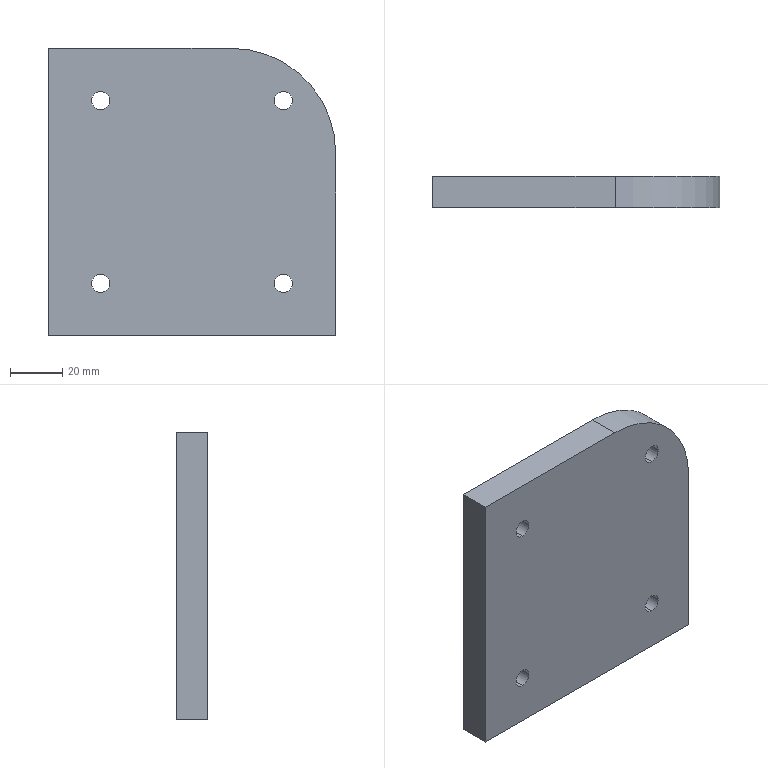Part | 1 solid | 15 faces | box 110 x 12 x 110 mm | volume 139232 mm3 | cylinder 9 | plane 6 | commonest cylinder face diameters 7 x8 80 x1
STEP:
#1=CARTESIAN_POINT('',(328.,-10.,546.5));
#2=VERTEX_POINT('',#1);
#3=CARTESIAN_POINT('',(328.,-10.,553.5));
#4=VERTEX_POINT('',#3);
#5=CARTESIAN_POINT('',(328.,-10.,550.));
#6=DIRECTION('',(0.,1.,0.));
#7=DIRECTION('',(0.,0.,1.));
#8=AXIS2_PLACEMENT_3D('',#5,#6,#7);
#9=CIRCLE('',#8,3.5);
#10=EDGE_CURVE('',#2,#4,#9,.T.);
#11=ORIENTED_EDGE('',*,*,#10,.F.);
#12=CARTESIAN_POINT('',(328.,2.,546.5));
#13=VERTEX_POINT('',#12);
#14=CARTESIAN_POINT('',(328.,-10.,546.5));
#15=DIRECTION('',(0.,1.,0.));
#16=VECTOR('',#15,1000.);
#17=LINE('',#14,#16);
#18=EDGE_CURVE('',#2,#13,#17,.T.);
#19=ORIENTED_EDGE('',*,*,#18,.T.);
#20=CARTESIAN_POINT('',(328.,2.,553.5));
#21=VERTEX_POINT('',#20);
#22=CARTESIAN_POINT('',(328.,2.,550.));
#23=DIRECTION('',(0.,-1.,0.));
#24=DIRECTION('',(0.,0.,1.));
#25=AXIS2_PLACEMENT_3D('',#22,#23,#24);
#26=CIRCLE('',#25,3.5);
#27=EDGE_CURVE('',#21,#13,#26,.T.);
#28=ORIENTED_EDGE('',*,*,#27,.F.);
#29=CARTESIAN_POINT('',(328.,-10.,553.5));
#30=DIRECTION('',(0.,1.,0.));
#31=VECTOR('',#30,1000.);
#32=LINE('',#29,#31);
#33=EDGE_CURVE('',#4,#21,#32,.T.);
#34=ORIENTED_EDGE('',*,*,#33,.F.);
#35=EDGE_LOOP('',(#11,#19,#28,#34));
#36=FACE_OUTER_BOUND('',#35,.T.);
#37=CARTESIAN_POINT('',(328.,-10.,550.));
#38=DIRECTION('',(0.,1.,0.));
#39=DIRECTION('',(0.,0.,1.));
#40=AXIS2_PLACEMENT_3D('',#37,#38,#39);
#41=CYLINDRICAL_SURFACE('',#40,3.5);
#42=ADVANCED_FACE('',(#36),#41,.F.);
#43=CARTESIAN_POINT('',(398.,-10.,546.5));
#44=VERTEX_POINT('',#43);
#45=CARTESIAN_POINT('',(398.,-10.,553.5));
#46=VERTEX_POINT('',#45);
#47=CARTESIAN_POINT('',(398.,-10.,550.));
#48=DIRECTION('',(0.,1.,0.));
#49=DIRECTION('',(0.,0.,1.));
#50=AXIS2_PLACEMENT_3D('',#47,#48,#49);
#51=CIRCLE('',#50,3.5);
#52=EDGE_CURVE('',#44,#46,#51,.T.);
#53=ORIENTED_EDGE('',*,*,#52,.F.);
#54=CARTESIAN_POINT('',(398.,2.,546.5));
#55=VERTEX_POINT('',#54);
#56=CARTESIAN_POINT('',(398.,-10.,546.5));
#57=DIRECTION('',(0.,1.,0.));
#58=VECTOR('',#57,1000.);
#59=LINE('',#56,#58);
#60=EDGE_CURVE('',#44,#55,#59,.T.);
#61=ORIENTED_EDGE('',*,*,#60,.T.);
#62=CARTESIAN_POINT('',(398.,2.,553.5));
#63=VERTEX_POINT('',#62);
#64=CARTESIAN_POINT('',(398.,2.,550.));
#65=DIRECTION('',(0.,-1.,0.));
#66=DIRECTION('',(0.,0.,1.));
#67=AXIS2_PLACEMENT_3D('',#64,#65,#66);
#68=CIRCLE('',#67,3.5);
#69=EDGE_CURVE('',#63,#55,#68,.T.);
#70=ORIENTED_EDGE('',*,*,#69,.F.);
#71=CARTESIAN_POINT('',(398.,-10.,553.5));
#72=DIRECTION('',(0.,1.,0.));
#73=VECTOR('',#72,1000.);
#74=LINE('',#71,#73);
#75=EDGE_CURVE('',#46,#63,#74,.T.);
#76=ORIENTED_EDGE('',*,*,#75,.F.);
#77=EDGE_LOOP('',(#53,#61,#70,#76));
#78=FACE_OUTER_BOUND('',#77,.T.);
#79=CARTESIAN_POINT('',(398.,-10.,550.));
#80=DIRECTION('',(0.,1.,0.));
#81=DIRECTION('',(0.,0.,1.));
#82=AXIS2_PLACEMENT_3D('',#79,#80,#81);
#83=CYLINDRICAL_SURFACE('',#82,3.5);
#84=ADVANCED_FACE('',(#78),#83,.F.);
#85=CARTESIAN_POINT('',(398.,-10.,616.5));
#86=VERTEX_POINT('',#85);
#87=CARTESIAN_POINT('',(398.,-10.,623.5));
#88=VERTEX_POINT('',#87);
#89=CARTESIAN_POINT('',(398.,-10.,620.));
#90=DIRECTION('',(0.,1.,0.));
#91=DIRECTION('',(0.,0.,1.));
#92=AXIS2_PLACEMENT_3D('',#89,#90,#91);
#93=CIRCLE('',#92,3.5);
#94=EDGE_CURVE('',#86,#88,#93,.T.);
#95=ORIENTED_EDGE('',*,*,#94,.F.);
#96=CARTESIAN_POINT('',(398.,2.,616.5));
#97=VERTEX_POINT('',#96);
#98=CARTESIAN_POINT('',(398.,-10.,616.5));
#99=DIRECTION('',(0.,1.,0.));
#100=VECTOR('',#99,1000.);
#101=LINE('',#98,#100);
#102=EDGE_CURVE('',#86,#97,#101,.T.);
#103=ORIENTED_EDGE('',*,*,#102,.T.);
#104=CARTESIAN_POINT('',(398.,2.,623.5));
#105=VERTEX_POINT('',#104);
#106=CARTESIAN_POINT('',(398.,2.,620.));
#107=DIRECTION('',(0.,-1.,0.));
#108=DIRECTION('',(0.,0.,1.));
#109=AXIS2_PLACEMENT_3D('',#106,#107,#108);
#110=CIRCLE('',#109,3.5);
#111=EDGE_CURVE('',#105,#97,#110,.T.);
#112=ORIENTED_EDGE('',*,*,#111,.F.);
#113=CARTESIAN_POINT('',(398.,-10.,623.5));
#114=DIRECTION('',(0.,1.,0.));
#115=VECTOR('',#114,1000.);
#116=LINE('',#113,#115);
#117=EDGE_CURVE('',#88,#105,#116,.T.);
#118=ORIENTED_EDGE('',*,*,#117,.F.);
#119=EDGE_LOOP('',(#95,#103,#112,#118));
#120=FACE_OUTER_BOUND('',#119,.T.);
#121=CARTESIAN_POINT('',(398.,-10.,620.));
#122=DIRECTION('',(0.,1.,0.));
#123=DIRECTION('',(0.,0.,1.));
#124=AXIS2_PLACEMENT_3D('',#121,#122,#123);
#125=CYLINDRICAL_SURFACE('',#124,3.5);
#126=ADVANCED_FACE('',(#120),#125,.F.);
#127=CARTESIAN_POINT('',(328.,-10.,616.5));
#128=VERTEX_POINT('',#127);
#129=CARTESIAN_POINT('',(328.,-10.,623.5));
#130=VERTEX_POINT('',#129);
#131=CARTESIAN_POINT('',(328.,-10.,620.));
#132=DIRECTION('',(0.,1.,0.));
#133=DIRECTION('',(0.,0.,1.));
#134=AXIS2_PLACEMENT_3D('',#131,#132,#133);
#135=CIRCLE('',#134,3.5);
#136=EDGE_CURVE('',#128,#130,#135,.T.);
#137=ORIENTED_EDGE('',*,*,#136,.F.);
#138=CARTESIAN_POINT('',(328.,2.,616.5));
#139=VERTEX_POINT('',#138);
#140=CARTESIAN_POINT('',(328.,-10.,616.5));
#141=DIRECTION('',(0.,1.,0.));
#142=VECTOR('',#141,1000.);
#143=LINE('',#140,#142);
#144=EDGE_CURVE('',#128,#139,#143,.T.);
#145=ORIENTED_EDGE('',*,*,#144,.T.);
#146=CARTESIAN_POINT('',(328.,2.,623.5));
#147=VERTEX_POINT('',#146);
#148=CARTESIAN_POINT('',(328.,2.,620.));
#149=DIRECTION('',(0.,-1.,0.));
#150=DIRECTION('',(0.,0.,1.));
#151=AXIS2_PLACEMENT_3D('',#148,#149,#150);
#152=CIRCLE('',#151,3.5);
#153=EDGE_CURVE('',#147,#139,#152,.T.);
#154=ORIENTED_EDGE('',*,*,#153,.F.);
#155=CARTESIAN_POINT('',(328.,-10.,623.5));
#156=DIRECTION('',(0.,1.,0.));
#157=VECTOR('',#156,1000.);
#158=LINE('',#155,#157);
#159=EDGE_CURVE('',#130,#147,#158,.T.);
#160=ORIENTED_EDGE('',*,*,#159,.F.);
#161=EDGE_LOOP('',(#137,#145,#154,#160));
#162=FACE_OUTER_BOUND('',#161,.T.);
#163=CARTESIAN_POINT('',(328.,-10.,620.));
#164=DIRECTION('',(0.,1.,0.));
#165=DIRECTION('',(0.,0.,1.));
#166=AXIS2_PLACEMENT_3D('',#163,#164,#165);
#167=CYLINDRICAL_SURFACE('',#166,3.5);
#168=ADVANCED_FACE('',(#162),#167,.F.);
#169=CARTESIAN_POINT('',(328.,-10.,550.));
#170=DIRECTION('',(0.,1.,0.));
#171=DIRECTION('',(0.,0.,1.));
#172=AXIS2_PLACEMENT_3D('',#169,#170,#171);
#173=CIRCLE('',#172,3.5);
#174=EDGE_CURVE('',#4,#2,#173,.T.);
#175=ORIENTED_EDGE('',*,*,#174,.T.);
#176=ORIENTED_EDGE('',*,*,#10,.T.);
#177=EDGE_LOOP('',(#175,#176));
#178=FACE_BOUND('',#177,.T.);
#179=CARTESIAN_POINT('',(398.,-10.,550.));
#180=DIRECTION('',(0.,1.,0.));
#181=DIRECTION('',(0.,0.,1.));
#182=AXIS2_PLACEMENT_3D('',#179,#180,#181);
#183=CIRCLE('',#182,3.5);
#184=EDGE_CURVE('',#46,#44,#183,.T.);
#185=ORIENTED_EDGE('',*,*,#184,.T.);
#186=ORIENTED_EDGE('',*,*,#52,.T.);
#187=EDGE_LOOP('',(#185,#186));
#188=FACE_BOUND('',#187,.T.);
#189=CARTESIAN_POINT('',(398.,-10.,620.));
#190=DIRECTION('',(0.,1.,0.));
#191=DIRECTION('',(0.,0.,1.));
#192=AXIS2_PLACEMENT_3D('',#189,#190,#191);
#193=CIRCLE('',#192,3.5);
#194=EDGE_CURVE('',#88,#86,#193,.T.);
#195=ORIENTED_EDGE('',*,*,#194,.T.);
#196=ORIENTED_EDGE('',*,*,#94,.T.);
#197=EDGE_LOOP('',(#195,#196));
#198=FACE_BOUND('',#197,.T.);
#199=CARTESIAN_POINT('',(328.,-10.,620.));
#200=DIRECTION('',(0.,1.,0.));
#201=DIRECTION('',(0.,0.,1.));
#202=AXIS2_PLACEMENT_3D('',#199,#200,#201);
#203=CIRCLE('',#202,3.5);
#204=EDGE_CURVE('',#130,#128,#203,.T.);
#205=ORIENTED_EDGE('',*,*,#204,.T.);
#206=ORIENTED_EDGE('',*,*,#136,.T.);
#207=EDGE_LOOP('',(#205,#206));
#208=FACE_BOUND('',#207,.T.);
#209=CARTESIAN_POINT('',(308.,-10.,640.));
#210=VERTEX_POINT('',#209);
#211=CARTESIAN_POINT('',(308.,-10.,530.));
#212=VERTEX_POINT('',#211);
#213=CARTESIAN_POINT('',(308.,-10.,80.));
#214=DIRECTION('',(0.,0.,-1.));
#215=VECTOR('',#214,1000.);
#216=LINE('',#213,#215);
#217=EDGE_CURVE('',#210,#212,#216,.T.);
#218=ORIENTED_EDGE('',*,*,#217,.T.);
#219=CARTESIAN_POINT('',(418.,-10.,530.));
#220=VERTEX_POINT('',#219);
#221=CARTESIAN_POINT('',(18.,-10.,530.));
#222=DIRECTION('',(1.,0.,0.));
#223=VECTOR('',#222,1000.);
#224=LINE('',#221,#223);
#225=EDGE_CURVE('',#212,#220,#224,.T.);
#226=ORIENTED_EDGE('',*,*,#225,.T.);
#227=CARTESIAN_POINT('',(418.,-10.,600.));
#228=VERTEX_POINT('',#227);
#229=CARTESIAN_POINT('',(418.,-10.,80.));
#230=DIRECTION('',(0.,0.,1.));
#231=VECTOR('',#230,1000.);
#232=LINE('',#229,#231);
#233=EDGE_CURVE('',#220,#228,#232,.T.);
#234=ORIENTED_EDGE('',*,*,#233,.T.);
#235=CARTESIAN_POINT('',(378.,-10.,640.));
#236=VERTEX_POINT('',#235);
#237=CARTESIAN_POINT('',(378.,-10.,600.));
#238=DIRECTION('',(0.,-1.,0.));
#239=DIRECTION('',(0.,0.,1.));
#240=AXIS2_PLACEMENT_3D('',#237,#238,#239);
#241=CIRCLE('',#240,40.);
#242=EDGE_CURVE('',#228,#236,#241,.T.);
#243=ORIENTED_EDGE('',*,*,#242,.T.);
#244=CARTESIAN_POINT('',(18.,-10.,640.));
#245=DIRECTION('',(-1.,0.,0.));
#246=VECTOR('',#245,1000.);
#247=LINE('',#244,#246);
#248=EDGE_CURVE('',#236,#210,#247,.T.);
#249=ORIENTED_EDGE('',*,*,#248,.T.);
#250=EDGE_LOOP('',(#218,#226,#234,#243,#249));
#251=FACE_OUTER_BOUND('',#250,.T.);
#252=CARTESIAN_POINT('',(18.,-10.,80.));
#253=DIRECTION('',(0.,-1.,0.));
#254=DIRECTION('',(0.,0.,-1.));
#255=AXIS2_PLACEMENT_3D('',#252,#253,#254);
#256=PLANE('',#255);
#257=ADVANCED_FACE('',(#178,#188,#198,#208,#251),#256,.T.);
#258=ORIENTED_EDGE('',*,*,#18,.F.);
#259=ORIENTED_EDGE('',*,*,#174,.F.);
#260=ORIENTED_EDGE('',*,*,#33,.T.);
#261=CARTESIAN_POINT('',(328.,2.,550.));
#262=DIRECTION('',(0.,-1.,0.));
#263=DIRECTION('',(0.,0.,1.));
#264=AXIS2_PLACEMENT_3D('',#261,#262,#263);
#265=CIRCLE('',#264,3.5);
#266=EDGE_CURVE('',#13,#21,#265,.T.);
#267=ORIENTED_EDGE('',*,*,#266,.F.);
#268=EDGE_LOOP('',(#258,#259,#260,#267));
#269=FACE_OUTER_BOUND('',#268,.T.);
#270=CARTESIAN_POINT('',(328.,-10.,550.));
#271=DIRECTION('',(0.,1.,0.));
#272=DIRECTION('',(0.,0.,1.));
#273=AXIS2_PLACEMENT_3D('',#270,#271,#272);
#274=CYLINDRICAL_SURFACE('',#273,3.5);
#275=ADVANCED_FACE('',(#269),#274,.F.);
#276=ORIENTED_EDGE('',*,*,#60,.F.);
#277=ORIENTED_EDGE('',*,*,#184,.F.);
#278=ORIENTED_EDGE('',*,*,#75,.T.);
#279=CARTESIAN_POINT('',(398.,2.,550.));
#280=DIRECTION('',(0.,-1.,0.));
#281=DIRECTION('',(0.,0.,1.));
#282=AXIS2_PLACEMENT_3D('',#279,#280,#281);
#283=CIRCLE('',#282,3.5);
#284=EDGE_CURVE('',#55,#63,#283,.T.);
#285=ORIENTED_EDGE('',*,*,#284,.F.);
#286=EDGE_LOOP('',(#276,#277,#278,#285));
#287=FACE_OUTER_BOUND('',#286,.T.);
#288=CARTESIAN_POINT('',(398.,-10.,550.));
#289=DIRECTION('',(0.,1.,0.));
#290=DIRECTION('',(0.,0.,1.));
#291=AXIS2_PLACEMENT_3D('',#288,#289,#290);
#292=CYLINDRICAL_SURFACE('',#291,3.5);
#293=ADVANCED_FACE('',(#287),#292,.F.);
#294=ORIENTED_EDGE('',*,*,#102,.F.);
#295=ORIENTED_EDGE('',*,*,#194,.F.);
#296=ORIENTED_EDGE('',*,*,#117,.T.);
#297=CARTESIAN_POINT('',(398.,2.,620.));
#298=DIRECTION('',(0.,-1.,0.));
#299=DIRECTION('',(0.,0.,1.));
#300=AXIS2_PLACEMENT_3D('',#297,#298,#299);
#301=CIRCLE('',#300,3.5);
#302=EDGE_CURVE('',#97,#105,#301,.T.);
#303=ORIENTED_EDGE('',*,*,#302,.F.);
#304=EDGE_LOOP('',(#294,#295,#296,#303));
#305=FACE_OUTER_BOUND('',#304,.T.);
#306=CARTESIAN_POINT('',(398.,-10.,620.));
#307=DIRECTION('',(0.,1.,0.));
#308=DIRECTION('',(0.,0.,1.));
#309=AXIS2_PLACEMENT_3D('',#306,#307,#308);
#310=CYLINDRICAL_SURFACE('',#309,3.5);
#311=ADVANCED_FACE('',(#305),#310,.F.);
#312=ORIENTED_EDGE('',*,*,#144,.F.);
#313=ORIENTED_EDGE('',*,*,#204,.F.);
#314=ORIENTED_EDGE('',*,*,#159,.T.);
#315=CARTESIAN_POINT('',(328.,2.,620.));
#316=DIRECTION('',(0.,-1.,0.));
#317=DIRECTION('',(0.,0.,1.));
#318=AXIS2_PLACEMENT_3D('',#315,#316,#317);
#319=CIRCLE('',#318,3.5);
#320=EDGE_CURVE('',#139,#147,#319,.T.);
#321=ORIENTED_EDGE('',*,*,#320,.F.);
#322=EDGE_LOOP('',(#312,#313,#314,#321));
#323=FACE_OUTER_BOUND('',#322,.T.);
#324=CARTESIAN_POINT('',(328.,-10.,620.));
#325=DIRECTION('',(0.,1.,0.));
#326=DIRECTION('',(0.,0.,1.));
#327=AXIS2_PLACEMENT_3D('',#324,#325,#326);
#328=CYLINDRICAL_SURFACE('',#327,3.5);
#329=ADVANCED_FACE('',(#323),#328,.F.);
#330=ORIENTED_EDGE('',*,*,#225,.F.);
#331=CARTESIAN_POINT('',(308.,2.,530.));
#332=VERTEX_POINT('',#331);
#333=CARTESIAN_POINT('',(308.,0.,530.));
#334=DIRECTION('',(0.,1.,0.));
#335=VECTOR('',#334,1000.);
#336=LINE('',#333,#335);
#337=EDGE_CURVE('',#212,#332,#336,.T.);
#338=ORIENTED_EDGE('',*,*,#337,.T.);
#339=CARTESIAN_POINT('',(418.,2.,530.));
#340=VERTEX_POINT('',#339);
#341=CARTESIAN_POINT('',(308.,2.,530.));
#342=DIRECTION('',(1.,0.,0.));
#343=VECTOR('',#342,1000.);
#344=LINE('',#341,#343);
#345=EDGE_CURVE('',#332,#340,#344,.T.);
#346=ORIENTED_EDGE('',*,*,#345,.T.);
#347=CARTESIAN_POINT('',(418.,0.,530.));
#348=DIRECTION('',(0.,-1.,0.));
#349=VECTOR('',#348,1000.);
#350=LINE('',#347,#349);
#351=EDGE_CURVE('',#340,#220,#350,.T.);
#352=ORIENTED_EDGE('',*,*,#351,.T.);
#353=EDGE_LOOP('',(#330,#338,#346,#352));
#354=FACE_OUTER_BOUND('',#353,.T.);
#355=CARTESIAN_POINT('',(308.,0.,530.));
#356=DIRECTION('',(0.,0.,-1.));
#357=DIRECTION('',(-1.,0.,0.));
#358=AXIS2_PLACEMENT_3D('',#355,#356,#357);
#359=PLANE('',#358);
#360=ADVANCED_FACE('',(#354),#359,.T.);
#361=ORIENTED_EDGE('',*,*,#217,.F.);
#362=CARTESIAN_POINT('',(308.,2.,640.));
#363=VERTEX_POINT('',#362);
#364=CARTESIAN_POINT('',(308.,0.,640.));
#365=DIRECTION('',(0.,1.,0.));
#366=VECTOR('',#365,1000.);
#367=LINE('',#364,#366);
#368=EDGE_CURVE('',#210,#363,#367,.T.);
#369=ORIENTED_EDGE('',*,*,#368,.T.);
#370=CARTESIAN_POINT('',(308.,2.,-150.));
#371=DIRECTION('',(0.,0.,-1.));
#372=VECTOR('',#371,1000.);
#373=LINE('',#370,#372);
#374=EDGE_CURVE('',#363,#332,#373,.T.);
#375=ORIENTED_EDGE('',*,*,#374,.T.);
#376=ORIENTED_EDGE('',*,*,#337,.F.);
#377=EDGE_LOOP('',(#361,#369,#375,#376));
#378=FACE_OUTER_BOUND('',#377,.T.);
#379=CARTESIAN_POINT('',(308.,0.,-150.));
#380=DIRECTION('',(-1.,0.,0.));
#381=DIRECTION('',(0.,0.,1.));
#382=AXIS2_PLACEMENT_3D('',#379,#380,#381);
#383=PLANE('',#382);
#384=ADVANCED_FACE('',(#378),#383,.T.);
#385=CARTESIAN_POINT('',(378.,2.,640.));
#386=VERTEX_POINT('',#385);
#387=CARTESIAN_POINT('',(378.,-10.,640.));
#388=DIRECTION('',(0.,-1.,0.));
#389=VECTOR('',#388,1000.);
#390=LINE('',#387,#389);
#391=EDGE_CURVE('',#386,#236,#390,.T.);
#392=ORIENTED_EDGE('',*,*,#391,.F.);
#393=CARTESIAN_POINT('',(418.,2.,640.));
#394=DIRECTION('',(1.,0.,0.));
#395=VECTOR('',#394,1000.);
#396=LINE('',#393,#395);
#397=EDGE_CURVE('',#363,#386,#396,.T.);
#398=ORIENTED_EDGE('',*,*,#397,.F.);
#399=ORIENTED_EDGE('',*,*,#368,.F.);
#400=ORIENTED_EDGE('',*,*,#248,.F.);
#401=EDGE_LOOP('',(#392,#398,#399,#400));
#402=FACE_OUTER_BOUND('',#401,.T.);
#403=CARTESIAN_POINT('',(418.,-10.,640.));
#404=DIRECTION('',(0.,0.,-1.));
#405=DIRECTION('',(-1.,0.,0.));
#406=AXIS2_PLACEMENT_3D('',#403,#404,#405);
#407=PLANE('',#406);
#408=ADVANCED_FACE('',(#402),#407,.F.);
#409=ORIENTED_EDGE('',*,*,#242,.F.);
#410=CARTESIAN_POINT('',(418.,2.,600.));
#411=VERTEX_POINT('',#410);
#412=CARTESIAN_POINT('',(418.,-10.,600.));
#413=DIRECTION('',(0.,1.,0.));
#414=VECTOR('',#413,1000.);
#415=LINE('',#412,#414);
#416=EDGE_CURVE('',#228,#411,#415,.T.);
#417=ORIENTED_EDGE('',*,*,#416,.T.);
#418=CARTESIAN_POINT('',(378.,2.,600.));
#419=DIRECTION('',(0.,-1.,0.));
#420=DIRECTION('',(0.,0.,1.));
#421=AXIS2_PLACEMENT_3D('',#418,#419,#420);
#422=CIRCLE('',#421,40.);
#423=EDGE_CURVE('',#411,#386,#422,.T.);
#424=ORIENTED_EDGE('',*,*,#423,.T.);
#425=ORIENTED_EDGE('',*,*,#391,.T.);
#426=EDGE_LOOP('',(#409,#417,#424,#425));
#427=FACE_OUTER_BOUND('',#426,.T.);
#428=CARTESIAN_POINT('',(378.,-10.,600.));
#429=DIRECTION('',(0.,1.,0.));
#430=DIRECTION('',(0.,0.,1.));
#431=AXIS2_PLACEMENT_3D('',#428,#429,#430);
#432=CYLINDRICAL_SURFACE('',#431,40.);
#433=ADVANCED_FACE('',(#427),#432,.T.);
#434=CARTESIAN_POINT('',(418.,2.,640.));
#435=DIRECTION('',(0.,0.,-1.));
#436=VECTOR('',#435,1000.);
#437=LINE('',#434,#436);
#438=EDGE_CURVE('',#411,#340,#437,.T.);
#439=ORIENTED_EDGE('',*,*,#438,.F.);
#440=ORIENTED_EDGE('',*,*,#416,.F.);
#441=ORIENTED_EDGE('',*,*,#233,.F.);
#442=ORIENTED_EDGE('',*,*,#351,.F.);
#443=EDGE_LOOP('',(#439,#440,#441,#442));
#444=FACE_OUTER_BOUND('',#443,.T.);
#445=CARTESIAN_POINT('',(418.,-10.,640.));
#446=DIRECTION('',(-1.,0.,0.));
#447=DIRECTION('',(0.,0.,1.));
#448=AXIS2_PLACEMENT_3D('',#445,#446,#447);
#449=PLANE('',#448);
#450=ADVANCED_FACE('',(#444),#449,.F.);
#451=ORIENTED_EDGE('',*,*,#27,.T.);
#452=ORIENTED_EDGE('',*,*,#266,.T.);
#453=EDGE_LOOP('',(#451,#452));
#454=FACE_BOUND('',#453,.T.);
#455=ORIENTED_EDGE('',*,*,#69,.T.);
#456=ORIENTED_EDGE('',*,*,#284,.T.);
#457=EDGE_LOOP('',(#455,#456));
#458=FACE_BOUND('',#457,.T.);
#459=ORIENTED_EDGE('',*,*,#111,.T.);
#460=ORIENTED_EDGE('',*,*,#302,.T.);
#461=EDGE_LOOP('',(#459,#460));
#462=FACE_BOUND('',#461,.T.);
#463=ORIENTED_EDGE('',*,*,#153,.T.);
#464=ORIENTED_EDGE('',*,*,#320,.T.);
#465=EDGE_LOOP('',(#463,#464));
#466=FACE_BOUND('',#465,.T.);
#467=ORIENTED_EDGE('',*,*,#397,.T.);
#468=ORIENTED_EDGE('',*,*,#423,.F.);
#469=ORIENTED_EDGE('',*,*,#438,.T.);
#470=ORIENTED_EDGE('',*,*,#345,.F.);
#471=ORIENTED_EDGE('',*,*,#374,.F.);
#472=EDGE_LOOP('',(#467,#468,#469,#470,#471));
#473=FACE_OUTER_BOUND('',#472,.T.);
#474=CARTESIAN_POINT('',(378.,2.,600.));
#475=DIRECTION('',(0.,1.,0.));
#476=DIRECTION('',(0.,0.,1.));
#477=AXIS2_PLACEMENT_3D('',#474,#475,#476);
#478=PLANE('',#477);
#479=ADVANCED_FACE('',(#454,#458,#462,#466,#473),#478,.T.);
#480=CLOSED_SHELL('',(#42,#84,#126,#168,#257,#275,#293,#311,#329,#360,#384,#408,#433,#450,#479));
#481=MANIFOLD_SOLID_BREP('',#480);
#482=CARTESIAN_POINT('',(0.,0.,0.));
#483=DIRECTION('',(0.,0.,1.));
#484=DIRECTION('',(1.,0.,0.));
#485=AXIS2_PLACEMENT_3D('',#482,#483,#484);
#486=(LENGTH_UNIT()NAMED_UNIT(*)SI_UNIT(.MILLI.,.METRE.));
#487=UNCERTAINTY_MEASURE_WITH_UNIT(LENGTH_MEASURE(0.00001),#486,'','');
#488=(NAMED_UNIT(*)PLANE_ANGLE_UNIT()SI_UNIT($,.RADIAN.));
#489=(NAMED_UNIT(*)SI_UNIT($,.STERADIAN.)SOLID_ANGLE_UNIT());
#490=(GEOMETRIC_REPRESENTATION_CONTEXT(3)GLOBAL_UNCERTAINTY_ASSIGNED_CONTEXT((#487))GLOBAL_UNIT_ASSIGNED_CONTEXT((#486,#488,#489))REPRESENTATION_CONTEXT('',''));
#491=ADVANCED_BREP_SHAPE_REPRESENTATION('',(#481,#485),#490);